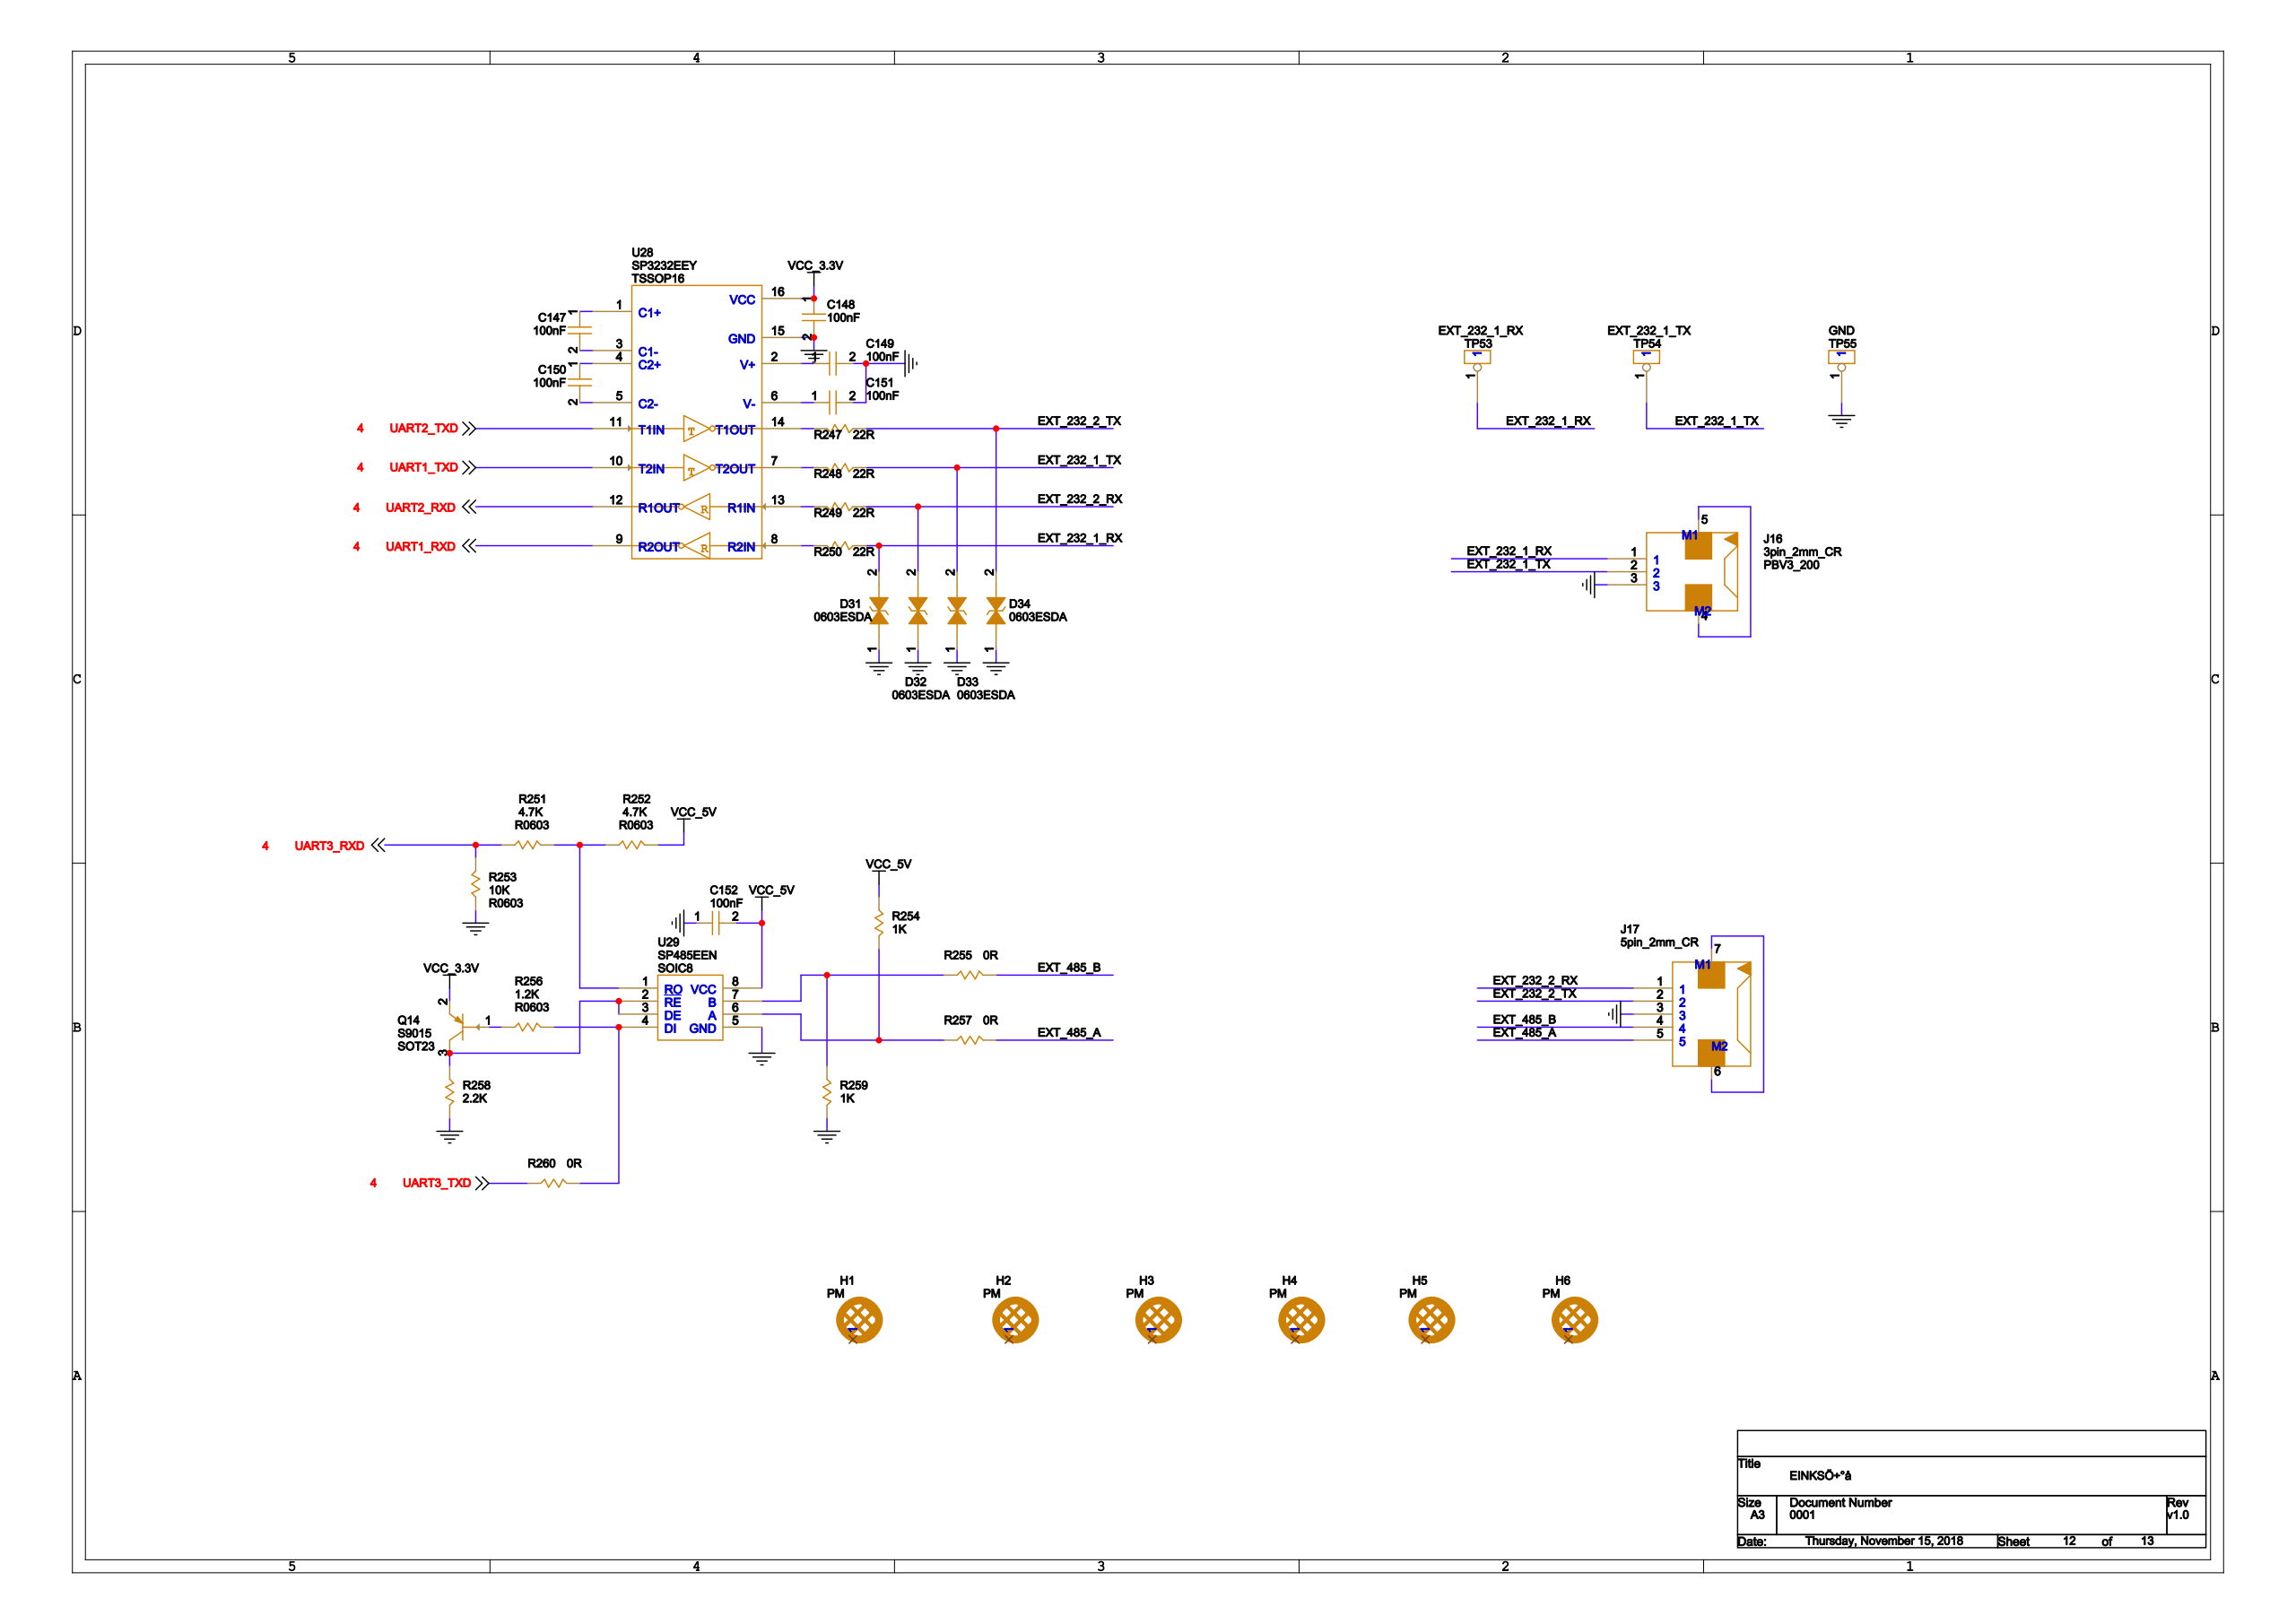Circuit board | Cadence Allegro | 609 parts | 409 nets | one sheet of the schematic
Parts on this sheet (reference | value | footprint):
C147 | 100nF | C0603
C148 | 100nF | C0603
C149 | 100nF | C0603
C150 | 100nF | C0603
C151 | 100nF | C0603
C152 | 100nF | C0603
D31 | 0603ESDA | 0603ESDA
D32 | 0603ESDA | 0603ESDA
D33 | 0603ESDA | 0603ESDA
D34 | 0603ESDA | 0603ESDA
J16 | 3pin_2mm_CR | PBV3_200
J17 | 5pin_2mm_CR | PBV5_200
Q14 | S9015 | SOT23
R247 | 22R | R0603
R248 | 22R | R0603
R249 | 22R | R0603
R250 | 22R | R0603
R251 | 4.7K | R0603
R252 | 4.7K | R0603
R253 | 10K | R0603
R254 | 1K | R0603
R255 | 0R | R0603
R256 | 1.2K | R0603
R257 | 0R | R0603
R258 | 2.2K | R0603
R259 | 1K | R0603
R260 | 0R | R0603
TP53 | EXT_232_1_RX | TP_50
TP54 | EXT_232_1_TX | TP_50
TP55 | GND | TP_50
U28 | SP3232EEY | TSSOP16
U29 | SP485EEN | SOIC8
Nets of these parts (net: part-pin ...):
GND: C148-2 C149-2 C151-2 C152-1 D31-1 D32-1 D33-1 D34-1 J16-3 J17-3 R253-1 R258-1 R259-2 TP55-1 U28-15 U29-5
VCC_3.3V: C148-1 Q14-2 U28-16
VCC_5V: C152-2 R252-1 R254-1 U29-8
EXT_232_1_RX: D31-2 J16-1 R250-2 TP53-1
EXT_232_1_TX: D33-2 J16-2 R248-2 TP54-1
N29161701: J16-4 J16-5
EXT_232_2_RX: D32-2 J17-1 R249-2
EXT_232_2_TX: D34-2 J17-2 R247-2
EXT_485_B: J17-4 R255-1
EXT_485_A: J17-5 R257-1
N29161818: J17-6 J17-7
UART1_RXD: U28-9
UART1_TXD: U28-10
UART2_RXD: U28-12
UART2_TXD: U28-11
UART3_RXD: R251-2 R253-2
UART3_TXD: R260-2
N29160580: Q14-1 R256-1
N29160515: Q14-3 R258-2 U29-2 U29-3
N29160517: R254-2 R257-2 U29-6
N29160554: R255-2 R259-1 U29-7
N29160594: R251-1 R252-2 U29-1
N29160479: R247-1 U28-14
N29160407: R248-1 U28-7
N29160471: R249-1 U28-13
N29160385: R250-1 U28-8
N29160552: R256-2 R260-1 U29-4
N29160409: C151-1 U28-6
N29160405: C147-1 U28-1
N29160403: C147-2 U28-3
N29160389: C149-1 U28-2
N29160401: C150-1 U28-4
N29160399: C150-2 U28-5